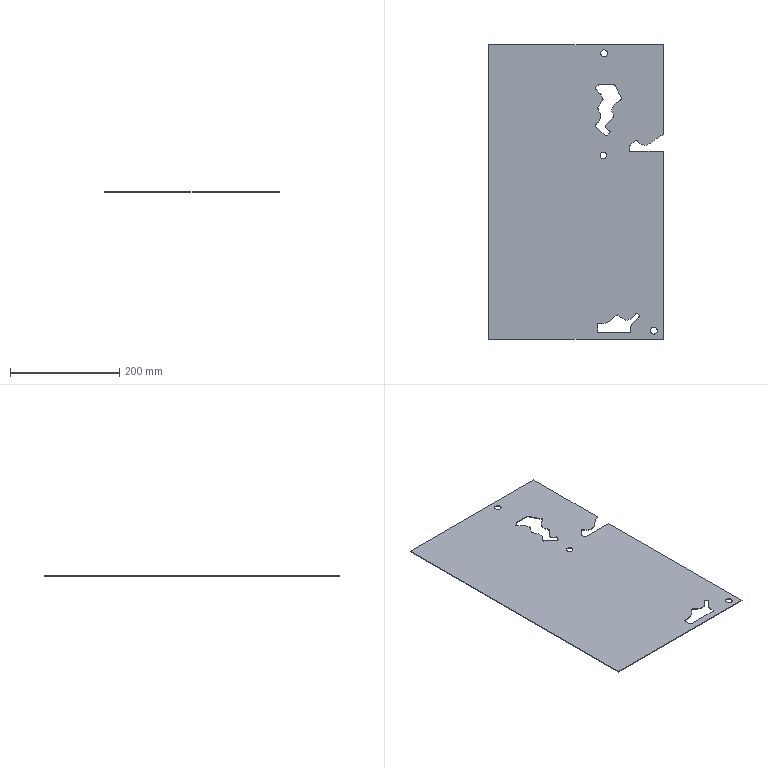Part | STEP file | gslz 2016.10.28-13_id150_x_t | 1 solid | 74 faces | box 319.858 x 540 x 1.25 mm | volume 209249 mm3 | cylinder 39 | plane 35 | commonest cylinder face diameters 4 x17 6 x4 10 x3 12.2 x2 20 x2 30 x2